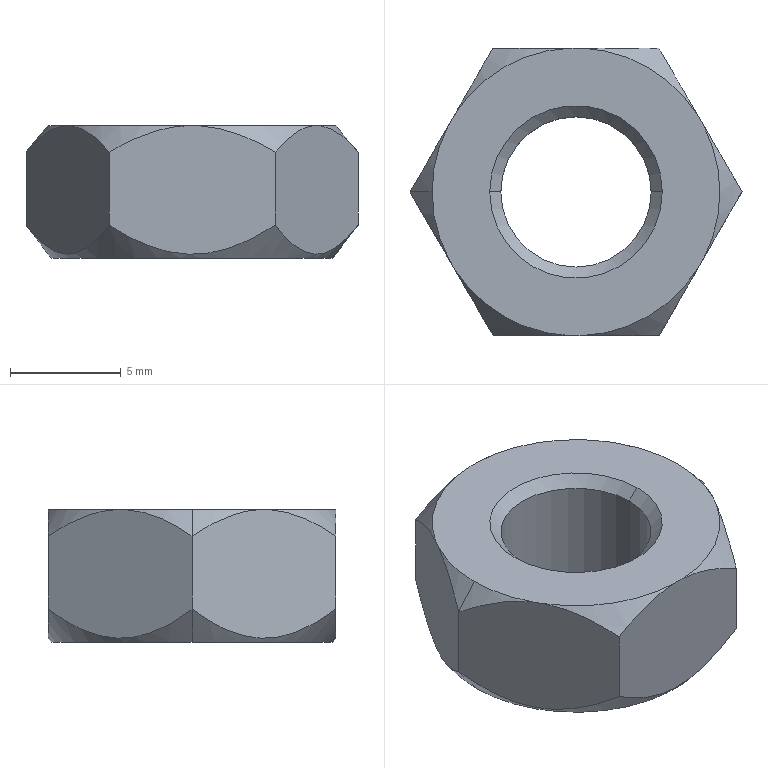Part | SolidWorks | features RevCut 3, Chamfer 2, Extrusion 1, RefAxis 1 | 1 solid | 23 faces | box 15.011 x 13.013 x 6 mm | volume 641.329 mm3 | cone 13 | plane 8 | cylinder 2 | commonest cylinder face diameters 6.8 x2
STEP:
#1=CARTESIAN_POINT('',(-3.4,0.,5.5));
#2=VERTEX_POINT('',#1);
#3=CARTESIAN_POINT('',(3.4,0.,5.5));
#4=VERTEX_POINT('',#3);
#5=CARTESIAN_POINT('',(0.,0.,5.5));
#6=DIRECTION('',(0.,0.,1.));
#7=DIRECTION('',(1.,0.,0.));
#8=AXIS2_PLACEMENT_3D('',#5,#6,#7);
#9=CIRCLE('',#8,3.4);
#10=EDGE_CURVE('',#2,#4,#9,.T.);
#11=ORIENTED_EDGE('',*,*,#10,.F.);
#12=CARTESIAN_POINT('',(-3.9,0.,6.));
#13=VERTEX_POINT('',#12);
#14=CARTESIAN_POINT('',(-3.4,0.,5.5));
#15=DIRECTION('',(-0.7071,0.,0.7071));
#16=VECTOR('',#15,1000.);
#17=LINE('',#14,#16);
#18=EDGE_CURVE('',#2,#13,#17,.T.);
#19=ORIENTED_EDGE('',*,*,#18,.T.);
#20=CARTESIAN_POINT('',(3.9,0.,6.));
#21=VERTEX_POINT('',#20);
#22=CARTESIAN_POINT('',(0.,0.,6.));
#23=DIRECTION('',(0.,0.,-1.));
#24=DIRECTION('',(1.,0.,0.));
#25=AXIS2_PLACEMENT_3D('',#22,#23,#24);
#26=CIRCLE('',#25,3.9);
#27=EDGE_CURVE('',#21,#13,#26,.T.);
#28=ORIENTED_EDGE('',*,*,#27,.F.);
#29=CARTESIAN_POINT('',(3.4,0.,5.5));
#30=DIRECTION('',(0.7071,0.,0.7071));
#31=VECTOR('',#30,1000.);
#32=LINE('',#29,#31);
#33=EDGE_CURVE('',#4,#21,#32,.T.);
#34=ORIENTED_EDGE('',*,*,#33,.F.);
#35=EDGE_LOOP('',(#11,#19,#28,#34));
#36=FACE_OUTER_BOUND('',#35,.T.);
#37=CARTESIAN_POINT('',(0.,0.,5.5));
#38=DIRECTION('',(0.,0.,1.));
#39=DIRECTION('',(1.,0.,0.));
#40=AXIS2_PLACEMENT_3D('',#37,#38,#39);
#41=CONICAL_SURFACE('',#40,3.4,0.7854);
#42=ADVANCED_FACE('',(#36),#41,.F.);
#43=CARTESIAN_POINT('',(3.4,0.,0.5));
#44=VERTEX_POINT('',#43);
#45=CARTESIAN_POINT('',(-3.4,0.,0.5));
#46=VERTEX_POINT('',#45);
#47=CARTESIAN_POINT('',(0.,0.,0.5));
#48=DIRECTION('',(0.,0.,-1.));
#49=DIRECTION('',(1.,0.,0.));
#50=AXIS2_PLACEMENT_3D('',#47,#48,#49);
#51=CIRCLE('',#50,3.4);
#52=EDGE_CURVE('',#44,#46,#51,.T.);
#53=ORIENTED_EDGE('',*,*,#52,.F.);
#54=CARTESIAN_POINT('',(3.9,0.,0.));
#55=VERTEX_POINT('',#54);
#56=CARTESIAN_POINT('',(3.9,0.,0.));
#57=DIRECTION('',(0.7071,0.,-0.7071));
#58=VECTOR('',#57,1000.);
#59=LINE('',#56,#58);
#60=EDGE_CURVE('',#44,#55,#59,.T.);
#61=ORIENTED_EDGE('',*,*,#60,.T.);
#62=CARTESIAN_POINT('',(-3.9,0.,0.));
#63=VERTEX_POINT('',#62);
#64=CARTESIAN_POINT('',(0.,0.,0.));
#65=DIRECTION('',(0.,0.,1.));
#66=DIRECTION('',(1.,0.,0.));
#67=AXIS2_PLACEMENT_3D('',#64,#65,#66);
#68=CIRCLE('',#67,3.9);
#69=EDGE_CURVE('',#63,#55,#68,.T.);
#70=ORIENTED_EDGE('',*,*,#69,.F.);
#71=CARTESIAN_POINT('',(-3.9,0.,0.));
#72=DIRECTION('',(-0.7071,0.,-0.7071));
#73=VECTOR('',#72,1000.);
#74=LINE('',#71,#73);
#75=EDGE_CURVE('',#46,#63,#74,.T.);
#76=ORIENTED_EDGE('',*,*,#75,.F.);
#77=EDGE_LOOP('',(#53,#61,#70,#76));
#78=FACE_OUTER_BOUND('',#77,.T.);
#79=CARTESIAN_POINT('',(0.,0.,0.));
#80=DIRECTION('',(0.,0.,-1.));
#81=DIRECTION('',(-1.,0.,0.));
#82=AXIS2_PLACEMENT_3D('',#79,#80,#81);
#83=CONICAL_SURFACE('',#82,3.9,0.7854);
#84=ADVANCED_FACE('',(#78),#83,.F.);
#85=CARTESIAN_POINT('',(-6.506,0.,6.));
#86=VERTEX_POINT('',#85);
#87=CARTESIAN_POINT('',(-5.758,-3.027,6.));
#88=VERTEX_POINT('',#87);
#89=CARTESIAN_POINT('',(0.,0.,6.));
#90=DIRECTION('',(0.,0.,1.));
#91=DIRECTION('',(1.,0.,0.));
#92=AXIS2_PLACEMENT_3D('',#89,#90,#91);
#93=CIRCLE('',#92,6.506);
#94=EDGE_CURVE('',#86,#88,#93,.T.);
#95=ORIENTED_EDGE('',*,*,#94,.F.);
#96=CARTESIAN_POINT('',(-7.498,0.,4.809));
#97=VERTEX_POINT('',#96);
#98=CARTESIAN_POINT('',(-6.506,0.,6.));
#99=DIRECTION('',(-0.6402,0.,-0.7682));
#100=VECTOR('',#99,1000.);
#101=LINE('',#98,#100);
#102=EDGE_CURVE('',#86,#97,#101,.T.);
#103=ORIENTED_EDGE('',*,*,#102,.T.);
#104=CARTESIAN_POINT('',(-7.506,-0.01301,4.8));
#105=VERTEX_POINT('',#104);
#106=CARTESIAN_POINT('',(-7.498,0.,4.809));
#107=CARTESIAN_POINT('',(-7.501,-0.004328,4.806));
#108=CARTESIAN_POINT('',(-7.503,-0.008655,4.803));
#109=CARTESIAN_POINT('',(-7.506,-0.01301,4.8));
#110=B_SPLINE_CURVE_WITH_KNOTS('',3,(#106,#107,#108,#109),.UNSPECIFIED.,.F.,.F.,(4,4),(0.01511,0.01513),.UNSPECIFIED.);
#111=EDGE_CURVE('',#97,#105,#110,.T.);
#112=ORIENTED_EDGE('',*,*,#111,.T.);
#113=CARTESIAN_POINT('',(-7.506,-0.01301,4.8));
#114=CARTESIAN_POINT('',(-7.373,-0.2423,4.959));
#115=CARTESIAN_POINT('',(-7.237,-0.4764,5.109));
#116=CARTESIAN_POINT('',(-6.958,-0.9577,5.384));
#117=CARTESIAN_POINT('',(-6.814,-1.206,5.509));
#118=CARTESIAN_POINT('',(-6.522,-1.71,5.723));
#119=CARTESIAN_POINT('',(-6.373,-1.966,5.811));
#120=CARTESIAN_POINT('',(-6.07,-2.489,5.942));
#121=CARTESIAN_POINT('',(-5.914,-2.759,5.985));
#122=CARTESIAN_POINT('',(-5.758,-3.027,6.));
#123=B_SPLINE_CURVE_WITH_KNOTS('',3,(#113,#114,#115,#116,#117,#118,#119,#120,#121,#122),.UNSPECIFIED.,.F.,.F.,(4,2,2,2,4),(0.007161,0.00809,0.00902,0.009949,0.01088),.UNSPECIFIED.);
#124=EDGE_CURVE('',#105,#88,#123,.T.);
#125=ORIENTED_EDGE('',*,*,#124,.T.);
#126=EDGE_LOOP('',(#95,#103,#112,#125));
#127=FACE_OUTER_BOUND('',#126,.T.);
#128=CARTESIAN_POINT('',(0.,0.,6.));
#129=DIRECTION('',(0.,0.,-1.));
#130=DIRECTION('',(-1.,0.,0.));
#131=AXIS2_PLACEMENT_3D('',#128,#129,#130);
#132=CONICAL_SURFACE('',#131,6.506,0.6947);
#133=ADVANCED_FACE('',(#127),#132,.T.);
#134=CARTESIAN_POINT('',(6.359,0.,0.));
#135=VERTEX_POINT('',#134);
#136=CARTESIAN_POINT('',(-6.359,0.,0.));
#137=VERTEX_POINT('',#136);
#138=CARTESIAN_POINT('',(0.,0.,0.));
#139=DIRECTION('',(0.,0.,1.));
#140=DIRECTION('',(1.,0.,0.));
#141=AXIS2_PLACEMENT_3D('',#138,#139,#140);
#142=CIRCLE('',#141,6.359);
#143=EDGE_CURVE('',#135,#137,#142,.T.);
#144=ORIENTED_EDGE('',*,*,#143,.T.);
#145=CARTESIAN_POINT('',(-7.498,0.,1.49));
#146=VERTEX_POINT('',#145);
#147=CARTESIAN_POINT('',(-7.506,0.,1.5));
#148=DIRECTION('',(-0.6074,0.,0.7944));
#149=VECTOR('',#148,1000.);
#150=LINE('',#147,#149);
#151=EDGE_CURVE('',#137,#146,#150,.T.);
#152=ORIENTED_EDGE('',*,*,#151,.T.);
#153=CARTESIAN_POINT('',(-3.764,6.493,1.5));
#154=VERTEX_POINT('',#153);
#155=CARTESIAN_POINT('',(-7.498,0.,1.49));
#156=CARTESIAN_POINT('',(-7.218,0.4875,1.124));
#157=CARTESIAN_POINT('',(-6.927,0.9929,0.8031));
#158=CARTESIAN_POINT('',(-6.463,1.8,0.4495));
#159=CARTESIAN_POINT('',(-6.303,2.079,0.3531));
#160=CARTESIAN_POINT('',(-5.972,2.654,0.22));
#161=CARTESIAN_POINT('',(-5.806,2.943,0.1855));
#162=CARTESIAN_POINT('',(-5.556,3.378,0.1847));
#163=CARTESIAN_POINT('',(-5.472,3.523,0.1928));
#164=CARTESIAN_POINT('',(-5.305,3.814,0.226));
#165=CARTESIAN_POINT('',(-5.221,3.96,0.2513));
#166=CARTESIAN_POINT('',(-4.974,4.39,0.3495));
#167=CARTESIAN_POINT('',(-4.814,4.668,0.4449));
#168=CARTESIAN_POINT('',(-4.5,5.214,0.6826));
#169=CARTESIAN_POINT('',(-4.346,5.481,0.8253));
#170=CARTESIAN_POINT('',(-4.049,5.997,1.141));
#171=CARTESIAN_POINT('',(-3.905,6.248,1.315));
#172=CARTESIAN_POINT('',(-3.764,6.493,1.5));
#173=B_SPLINE_CURVE_WITH_KNOTS('',3,(#155,#156,#157,#158,#159,#160,#161,#162,#163,#164,#165,#166,#167,#168,#169,#170,#171,#172),.UNSPECIFIED.,.F.,.F.,(4,2,2,2,2,2,2,2,4),(0.00001801,0.002007,0.003001,0.003996,0.004493,0.00499,0.005985,0.006979,0.007974),.UNSPECIFIED.);
#174=EDGE_CURVE('',#146,#154,#173,.T.);
#175=ORIENTED_EDGE('',*,*,#174,.T.);
#176=CARTESIAN_POINT('',(3.742,6.506,1.5));
#177=VERTEX_POINT('',#176);
#178=CARTESIAN_POINT('',(-3.764,6.493,1.5));
#179=CARTESIAN_POINT('',(-3.201,6.494,1.132));
#180=CARTESIAN_POINT('',(-2.617,6.495,0.8095));
#181=CARTESIAN_POINT('',(-1.684,6.497,0.4534));
#182=CARTESIAN_POINT('',(-1.363,6.498,0.3562));
#183=CARTESIAN_POINT('',(-0.6975,6.499,0.2214));
#184=CARTESIAN_POINT('',(-0.3636,6.499,0.1861));
#185=CARTESIAN_POINT('',(0.1388,6.5,0.1844));
#186=CARTESIAN_POINT('',(0.3066,6.501,0.1923));
#187=CARTESIAN_POINT('',(0.6427,6.501,0.225));
#188=CARTESIAN_POINT('',(0.8115,6.501,0.2501));
#189=CARTESIAN_POINT('',(1.309,6.502,0.3479));
#190=CARTESIAN_POINT('',(1.631,6.503,0.4433));
#191=CARTESIAN_POINT('',(2.262,6.504,0.681));
#192=CARTESIAN_POINT('',(2.571,6.504,0.824));
#193=CARTESIAN_POINT('',(3.168,6.506,1.141));
#194=CARTESIAN_POINT('',(3.458,6.506,1.315));
#195=CARTESIAN_POINT('',(3.742,6.506,1.5));
#196=B_SPLINE_CURVE_WITH_KNOTS('',3,(#178,#179,#180,#181,#182,#183,#184,#185,#186,#187,#188,#189,#190,#191,#192,#193,#194,#195),.UNSPECIFIED.,.F.,.F.,(4,2,2,2,2,2,2,2,4),(0.000000361,0.001994,0.00299,0.003987,0.004486,0.004984,0.005981,0.006977,0.007974),.UNSPECIFIED.);
#197=EDGE_CURVE('',#154,#177,#196,.T.);
#198=ORIENTED_EDGE('',*,*,#197,.T.);
#199=CARTESIAN_POINT('',(7.506,0.01301,1.5));
#200=VERTEX_POINT('',#199);
#201=CARTESIAN_POINT('',(3.742,6.506,1.5));
#202=CARTESIAN_POINT('',(4.024,6.019,1.132));
#203=CARTESIAN_POINT('',(4.317,5.514,0.8095));
#204=CARTESIAN_POINT('',(4.784,4.707,0.4534));
#205=CARTESIAN_POINT('',(4.946,4.429,0.3562));
#206=CARTESIAN_POINT('',(5.279,3.853,0.2214));
#207=CARTESIAN_POINT('',(5.447,3.565,0.1861));
#208=CARTESIAN_POINT('',(5.699,3.13,0.1844));
#209=CARTESIAN_POINT('',(5.783,2.985,0.1923));
#210=CARTESIAN_POINT('',(5.951,2.694,0.225));
#211=CARTESIAN_POINT('',(6.036,2.548,0.2501));
#212=CARTESIAN_POINT('',(6.286,2.118,0.3479));
#213=CARTESIAN_POINT('',(6.447,1.839,0.4433));
#214=CARTESIAN_POINT('',(6.763,1.293,0.681));
#215=CARTESIAN_POINT('',(6.918,1.026,0.824));
#216=CARTESIAN_POINT('',(7.218,0.5092,1.141));
#217=CARTESIAN_POINT('',(7.363,0.2584,1.315));
#218=CARTESIAN_POINT('',(7.506,0.01301,1.5));
#219=B_SPLINE_CURVE_WITH_KNOTS('',3,(#201,#202,#203,#204,#205,#206,#207,#208,#209,#210,#211,#212,#213,#214,#215,#216,#217,#218),.UNSPECIFIED.,.F.,.F.,(4,2,2,2,2,2,2,2,4),(0.000000361,0.001994,0.00299,0.003987,0.004486,0.004984,0.005981,0.006977,0.007974),.UNSPECIFIED.);
#220=EDGE_CURVE('',#177,#200,#219,.T.);
#221=ORIENTED_EDGE('',*,*,#220,.T.);
#222=CARTESIAN_POINT('',(7.498,0.,1.49));
#223=VERTEX_POINT('',#222);
#224=CARTESIAN_POINT('',(7.506,0.01301,1.5));
#225=CARTESIAN_POINT('',(7.503,0.008651,1.497));
#226=CARTESIAN_POINT('',(7.501,0.004326,1.493));
#227=CARTESIAN_POINT('',(7.498,0.,1.49));
#228=B_SPLINE_CURVE_WITH_KNOTS('',3,(#224,#225,#226,#227),.UNSPECIFIED.,.F.,.F.,(4,4),(0.000000361,0.00001801),.UNSPECIFIED.);
#229=EDGE_CURVE('',#200,#223,#228,.T.);
#230=ORIENTED_EDGE('',*,*,#229,.T.);
#231=CARTESIAN_POINT('',(7.506,0.,1.5));
#232=DIRECTION('',(0.6074,0.,0.7944));
#233=VECTOR('',#232,1000.);
#234=LINE('',#231,#233);
#235=EDGE_CURVE('',#135,#223,#234,.T.);
#236=ORIENTED_EDGE('',*,*,#235,.F.);
#237=EDGE_LOOP('',(#144,#152,#175,#198,#221,#230,#236));
#238=FACE_OUTER_BOUND('',#237,.T.);
#239=CARTESIAN_POINT('',(0.,0.,1.5));
#240=DIRECTION('',(0.,0.,1.));
#241=DIRECTION('',(1.,0.,0.));
#242=AXIS2_PLACEMENT_3D('',#239,#240,#241);
#243=CONICAL_SURFACE('',#242,7.506,0.6528);
#244=ADVANCED_FACE('',(#238),#243,.T.);
#245=ORIENTED_EDGE('',*,*,#10,.T.);
#246=CARTESIAN_POINT('',(3.4,0.,6.));
#247=DIRECTION('',(0.,0.,-1.));
#248=VECTOR('',#247,1000.);
#249=LINE('',#246,#248);
#250=EDGE_CURVE('',#4,#44,#249,.T.);
#251=ORIENTED_EDGE('',*,*,#250,.T.);
#252=ORIENTED_EDGE('',*,*,#52,.T.);
#253=CARTESIAN_POINT('',(-3.4,0.,6.));
#254=DIRECTION('',(0.,0.,-1.));
#255=VECTOR('',#254,1000.);
#256=LINE('',#253,#255);
#257=EDGE_CURVE('',#2,#46,#256,.T.);
#258=ORIENTED_EDGE('',*,*,#257,.F.);
#259=EDGE_LOOP('',(#245,#251,#252,#258));
#260=FACE_OUTER_BOUND('',#259,.T.);
#261=CARTESIAN_POINT('',(0.,0.,6.));
#262=DIRECTION('',(0.,0.,-1.));
#263=DIRECTION('',(-1.,0.,0.));
#264=AXIS2_PLACEMENT_3D('',#261,#262,#263);
#265=CYLINDRICAL_SURFACE('',#264,3.4);
#266=ADVANCED_FACE('',(#260),#265,.F.);
#267=ORIENTED_EDGE('',*,*,#124,.F.);
#268=CARTESIAN_POINT('',(-7.506,-0.01301,1.5));
#269=VERTEX_POINT('',#268);
#270=CARTESIAN_POINT('',(-7.506,-0.01301,6.));
#271=DIRECTION('',(0.,0.,-1.));
#272=VECTOR('',#271,1000.);
#273=LINE('',#270,#272);
#274=EDGE_CURVE('',#105,#269,#273,.T.);
#275=ORIENTED_EDGE('',*,*,#274,.T.);
#276=CARTESIAN_POINT('',(-3.742,-6.506,1.5));
#277=VERTEX_POINT('',#276);
#278=CARTESIAN_POINT('',(-3.742,-6.506,1.5));
#279=CARTESIAN_POINT('',(-4.024,-6.019,1.132));
#280=CARTESIAN_POINT('',(-4.317,-5.514,0.8095));
#281=CARTESIAN_POINT('',(-4.784,-4.707,0.4534));
#282=CARTESIAN_POINT('',(-4.946,-4.429,0.3562));
#283=CARTESIAN_POINT('',(-5.279,-3.853,0.2214));
#284=CARTESIAN_POINT('',(-5.447,-3.565,0.1861));
#285=CARTESIAN_POINT('',(-5.699,-3.13,0.1844));
#286=CARTESIAN_POINT('',(-5.783,-2.985,0.1923));
#287=CARTESIAN_POINT('',(-5.951,-2.694,0.225));
#288=CARTESIAN_POINT('',(-6.036,-2.548,0.2501));
#289=CARTESIAN_POINT('',(-6.286,-2.118,0.3479));
#290=CARTESIAN_POINT('',(-6.447,-1.839,0.4433));
#291=CARTESIAN_POINT('',(-6.763,-1.293,0.681));
#292=CARTESIAN_POINT('',(-6.918,-1.026,0.824));
#293=CARTESIAN_POINT('',(-7.218,-0.5092,1.141));
#294=CARTESIAN_POINT('',(-7.363,-0.2584,1.315));
#295=CARTESIAN_POINT('',(-7.506,-0.01301,1.5));
#296=B_SPLINE_CURVE_WITH_KNOTS('',3,(#278,#279,#280,#281,#282,#283,#284,#285,#286,#287,#288,#289,#290,#291,#292,#293,#294,#295),.UNSPECIFIED.,.F.,.F.,(4,2,2,2,2,2,2,2,4),(0.000000361,0.001994,0.00299,0.003987,0.004486,0.004984,0.005981,0.006977,0.007974),.UNSPECIFIED.);
#297=EDGE_CURVE('',#277,#269,#296,.T.);
#298=ORIENTED_EDGE('',*,*,#297,.F.);
#299=CARTESIAN_POINT('',(-3.742,-6.506,4.8));
#300=VERTEX_POINT('',#299);
#301=CARTESIAN_POINT('',(-3.742,-6.506,6.));
#302=DIRECTION('',(0.,0.,-1.));
#303=VECTOR('',#302,1000.);
#304=LINE('',#301,#303);
#305=EDGE_CURVE('',#300,#277,#304,.T.);
#306=ORIENTED_EDGE('',*,*,#305,.F.);
#307=CARTESIAN_POINT('',(-5.489,-3.492,6.));
#308=VERTEX_POINT('',#307);
#309=CARTESIAN_POINT('',(-5.489,-3.492,6.));
#310=CARTESIAN_POINT('',(-5.334,-3.759,5.985));
#311=CARTESIAN_POINT('',(-5.18,-4.024,5.943));
#312=CARTESIAN_POINT('',(-4.875,-4.55,5.812));
#313=CARTESIAN_POINT('',(-4.724,-4.812,5.722));
#314=CARTESIAN_POINT('',(-4.285,-5.568,5.401));
#315=CARTESIAN_POINT('',(-4.009,-6.045,5.12));
#316=CARTESIAN_POINT('',(-3.742,-6.506,4.8));
#317=B_SPLINE_CURVE_WITH_KNOTS('',3,(#309,#310,#311,#312,#313,#314,#315,#316),.UNSPECIFIED.,.F.,.F.,(4,2,2,4),(0.01142,0.01235,0.01328,0.01515),.UNSPECIFIED.);
#318=EDGE_CURVE('',#308,#300,#317,.T.);
#319=ORIENTED_EDGE('',*,*,#318,.F.);
#320=CARTESIAN_POINT('',(-7.506,-0.01301,6.));
#321=DIRECTION('',(0.5015,-0.8652,0.));
#322=VECTOR('',#321,1000.);
#323=LINE('',#320,#322);
#324=EDGE_CURVE('',#88,#308,#323,.T.);
#325=ORIENTED_EDGE('',*,*,#324,.F.);
#326=EDGE_LOOP('',(#267,#275,#298,#306,#319,#325));
#327=FACE_OUTER_BOUND('',#326,.T.);
#328=CARTESIAN_POINT('',(-7.506,-0.01301,6.));
#329=DIRECTION('',(0.8652,0.5015,0.));
#330=DIRECTION('',(-0.5015,0.8652,0.));
#331=AXIS2_PLACEMENT_3D('',#328,#329,#330);
#332=PLANE('',#331);
#333=ADVANCED_FACE('',(#327),#332,.F.);
#334=CARTESIAN_POINT('',(-0.2572,-6.5,6.));
#335=VERTEX_POINT('',#334);
#336=CARTESIAN_POINT('',(-3.742,-6.506,4.8));
#337=CARTESIAN_POINT('',(-3.207,-6.506,5.12));
#338=CARTESIAN_POINT('',(-2.655,-6.505,5.402));
#339=CARTESIAN_POINT('',(-1.78,-6.503,5.723));
#340=CARTESIAN_POINT('',(-1.478,-6.503,5.812));
#341=CARTESIAN_POINT('',(-0.8727,-6.502,5.943));
#342=CARTESIAN_POINT('',(-0.5667,-6.501,5.985));
#343=CARTESIAN_POINT('',(-0.2572,-6.5,6.));
#344=B_SPLINE_CURVE_WITH_KNOTS('',3,(#336,#337,#338,#339,#340,#341,#342,#343),.UNSPECIFIED.,.F.,.F.,(4,2,2,4),(0.005934,0.007788,0.008715,0.009642),.UNSPECIFIED.);
#345=EDGE_CURVE('',#300,#335,#344,.T.);
#346=ORIENTED_EDGE('',*,*,#345,.F.);
#347=ORIENTED_EDGE('',*,*,#305,.T.);
#348=CARTESIAN_POINT('',(3.764,-6.493,1.5));
#349=VERTEX_POINT('',#348);
#350=CARTESIAN_POINT('',(3.764,-6.493,1.5));
#351=CARTESIAN_POINT('',(3.201,-6.494,1.132));
#352=CARTESIAN_POINT('',(2.617,-6.495,0.8095));
#353=CARTESIAN_POINT('',(1.684,-6.497,0.4534));
#354=CARTESIAN_POINT('',(1.363,-6.498,0.3562));
#355=CARTESIAN_POINT('',(0.6975,-6.499,0.2214));
#356=CARTESIAN_POINT('',(0.3636,-6.499,0.1861));
#357=CARTESIAN_POINT('',(-0.1388,-6.5,0.1844));
#358=CARTESIAN_POINT('',(-0.3066,-6.501,0.1923));
#359=CARTESIAN_POINT('',(-0.6427,-6.501,0.225));
#360=CARTESIAN_POINT('',(-0.8115,-6.501,0.2501));
#361=CARTESIAN_POINT('',(-1.309,-6.502,0.3479));
#362=CARTESIAN_POINT('',(-1.631,-6.503,0.4433));
#363=CARTESIAN_POINT('',(-2.262,-6.504,0.681));
#364=CARTESIAN_POINT('',(-2.571,-6.504,0.824));
#365=CARTESIAN_POINT('',(-3.168,-6.506,1.141));
#366=CARTESIAN_POINT('',(-3.458,-6.506,1.315));
#367=CARTESIAN_POINT('',(-3.742,-6.506,1.5));
#368=B_SPLINE_CURVE_WITH_KNOTS('',3,(#350,#351,#352,#353,#354,#355,#356,#357,#358,#359,#360,#361,#362,#363,#364,#365,#366,#367),.UNSPECIFIED.,.F.,.F.,(4,2,2,2,2,2,2,2,4),(0.000000361,0.001994,0.00299,0.003987,0.004486,0.004984,0.005981,0.006977,0.007974),.UNSPECIFIED.);
#369=EDGE_CURVE('',#349,#277,#368,.T.);
#370=ORIENTED_EDGE('',*,*,#369,.F.);
#371=CARTESIAN_POINT('',(3.764,-6.493,4.8));
#372=VERTEX_POINT('',#371);
#373=CARTESIAN_POINT('',(3.764,-6.493,6.));
#374=DIRECTION('',(0.,0.,-1.));
#375=VECTOR('',#374,1000.);
#376=LINE('',#373,#375);
#377=EDGE_CURVE('',#372,#349,#376,.T.);
#378=ORIENTED_EDGE('',*,*,#377,.F.);
#379=CARTESIAN_POINT('',(0.2797,-6.5,6.));
#380=VERTEX_POINT('',#379);
#381=CARTESIAN_POINT('',(0.2797,-6.5,6.));
#382=CARTESIAN_POINT('',(0.9057,-6.498,5.969));
#383=CARTESIAN_POINT('',(1.509,-6.497,5.83));
#384=CARTESIAN_POINT('',(2.684,-6.495,5.4));
#385=CARTESIAN_POINT('',(3.234,-6.494,5.118));
#386=CARTESIAN_POINT('',(3.764,-6.493,4.8));
#387=B_SPLINE_CURVE_WITH_KNOTS('',3,(#381,#382,#383,#384,#385,#386),.UNSPECIFIED.,.F.,.F.,(4,2,4),(0.01017,0.01203,0.01389),.UNSPECIFIED.);
#388=EDGE_CURVE('',#380,#372,#387,.T.);
#389=ORIENTED_EDGE('',*,*,#388,.F.);
#390=CARTESIAN_POINT('',(-3.742,-6.506,6.));
#391=DIRECTION('',(1.,0.001733,0.));
#392=VECTOR('',#391,1000.);
#393=LINE('',#390,#392);
#394=EDGE_CURVE('',#335,#380,#393,.T.);
#395=ORIENTED_EDGE('',*,*,#394,.F.);
#396=EDGE_LOOP('',(#346,#347,#370,#378,#389,#395));
#397=FACE_OUTER_BOUND('',#396,.T.);
#398=CARTESIAN_POINT('',(-3.742,-6.506,6.));
#399=DIRECTION('',(-0.001733,1.,0.));
#400=DIRECTION('',(-1.,-0.001733,0.));
#401=AXIS2_PLACEMENT_3D('',#398,#399,#400);
#402=PLANE('',#401);
#403=ADVANCED_FACE('',(#397),#402,.F.);
#404=CARTESIAN_POINT('',(5.501,-3.473,6.));
#405=VERTEX_POINT('',#404);
#406=CARTESIAN_POINT('',(3.764,-6.493,4.8));
#407=CARTESIAN_POINT('',(3.896,-6.264,4.959));
#408=CARTESIAN_POINT('',(4.031,-6.029,5.109));
#409=CARTESIAN_POINT('',(4.308,-5.547,5.384));
#410=CARTESIAN_POINT('',(4.452,-5.298,5.509));
#411=CARTESIAN_POINT('',(4.742,-4.793,5.723));
#412=CARTESIAN_POINT('',(4.889,-4.536,5.811));
#413=CARTESIAN_POINT('',(5.191,-4.012,5.942));
#414=CARTESIAN_POINT('',(5.346,-3.742,5.985));
#415=CARTESIAN_POINT('',(5.501,-3.473,6.));
#416=B_SPLINE_CURVE_WITH_KNOTS('',3,(#406,#407,#408,#409,#410,#411,#412,#413,#414,#415),.UNSPECIFIED.,.F.,.F.,(4,2,2,2,4),(0.007144,0.008073,0.009002,0.009932,0.01086),.UNSPECIFIED.);
#417=EDGE_CURVE('',#372,#405,#416,.T.);
#418=ORIENTED_EDGE('',*,*,#417,.F.);
#419=ORIENTED_EDGE('',*,*,#377,.T.);
#420=CARTESIAN_POINT('',(7.498,0.,1.49));
#421=CARTESIAN_POINT('',(7.218,-0.4875,1.124));
#422=CARTESIAN_POINT('',(6.927,-0.9929,0.8031));
#423=CARTESIAN_POINT('',(6.463,-1.8,0.4495));
#424=CARTESIAN_POINT('',(6.303,-2.079,0.3531));
#425=CARTESIAN_POINT('',(5.972,-2.654,0.22));
#426=CARTESIAN_POINT('',(5.806,-2.943,0.1855));
#427=CARTESIAN_POINT('',(5.556,-3.378,0.1847));
#428=CARTESIAN_POINT('',(5.472,-3.523,0.1928));
#429=CARTESIAN_POINT('',(5.305,-3.814,0.226));
#430=CARTESIAN_POINT('',(5.221,-3.96,0.2513));
#431=CARTESIAN_POINT('',(4.974,-4.39,0.3495));
#432=CARTESIAN_POINT('',(4.814,-4.668,0.4449));
#433=CARTESIAN_POINT('',(4.5,-5.214,0.6826));
#434=CARTESIAN_POINT('',(4.346,-5.481,0.8253));
#435=CARTESIAN_POINT('',(4.049,-5.997,1.141));
#436=CARTESIAN_POINT('',(3.905,-6.248,1.315));
#437=CARTESIAN_POINT('',(3.764,-6.493,1.5));
#438=B_SPLINE_CURVE_WITH_KNOTS('',3,(#420,#421,#422,#423,#424,#425,#426,#427,#428,#429,#430,#431,#432,#433,#434,#435,#436,#437),.UNSPECIFIED.,.F.,.F.,(4,2,2,2,2,2,2,2,4),(0.00001801,0.002007,0.003001,0.003996,0.004493,0.00499,0.005985,0.006979,0.007974),.UNSPECIFIED.);
#439=EDGE_CURVE('',#223,#349,#438,.T.);
#440=ORIENTED_EDGE('',*,*,#439,.F.);
#441=ORIENTED_EDGE('',*,*,#229,.F.);
#442=CARTESIAN_POINT('',(7.506,0.01301,4.8));
#443=VERTEX_POINT('',#442);
#444=CARTESIAN_POINT('',(7.506,0.01301,6.));
#445=DIRECTION('',(0.,0.,-1.));
#446=VECTOR('',#445,1000.);
#447=LINE('',#444,#446);
#448=EDGE_CURVE('',#443,#200,#447,.T.);
#449=ORIENTED_EDGE('',*,*,#448,.F.);
#450=CARTESIAN_POINT('',(5.769,-3.007,6.));
#451=VERTEX_POINT('',#450);
#452=CARTESIAN_POINT('',(5.769,-3.007,6.));
#453=CARTESIAN_POINT('',(5.923,-2.74,5.985));
#454=CARTESIAN_POINT('',(6.075,-2.474,5.943));
#455=CARTESIAN_POINT('',(6.378,-1.947,5.812));
#456=CARTESIAN_POINT('',(6.529,-1.685,5.722));
#457=CARTESIAN_POINT('',(6.965,-0.9271,5.401));
#458=CARTESIAN_POINT('',(7.24,-0.4492,5.12));
#459=CARTESIAN_POINT('',(7.506,0.01301,4.8));
#460=B_SPLINE_CURVE_WITH_KNOTS('',3,(#452,#453,#454,#455,#456,#457,#458,#459),.UNSPECIFIED.,.F.,.F.,(4,2,2,4),(0.0114,0.01233,0.01326,0.01513),.UNSPECIFIED.);
#461=EDGE_CURVE('',#451,#443,#460,.T.);
#462=ORIENTED_EDGE('',*,*,#461,.F.);
#463=CARTESIAN_POINT('',(3.764,-6.493,6.));
#464=DIRECTION('',(0.4985,0.8669,0.));
#465=VECTOR('',#464,1000.);
#466=LINE('',#463,#465);
#467=EDGE_CURVE('',#405,#451,#466,.T.);
#468=ORIENTED_EDGE('',*,*,#467,.F.);
#469=EDGE_LOOP('',(#418,#419,#440,#441,#449,#462,#468));
#470=FACE_OUTER_BOUND('',#469,.T.);
#471=CARTESIAN_POINT('',(3.764,-6.493,6.));
#472=DIRECTION('',(-0.8669,0.4985,0.));
#473=DIRECTION('',(-0.4985,-0.8669,0.));
#474=AXIS2_PLACEMENT_3D('',#471,#472,#473);
#475=PLANE('',#474);
#476=ADVANCED_FACE('',(#470),#475,.F.);
#477=CARTESIAN_POINT('',(5.758,3.027,6.));
#478=VERTEX_POINT('',#477);
#479=CARTESIAN_POINT('',(7.506,0.01301,4.8));
#480=CARTESIAN_POINT('',(7.373,0.2423,4.959));
#481=CARTESIAN_POINT('',(7.237,0.4764,5.109));
#482=CARTESIAN_POINT('',(6.958,0.9577,5.384));
#483=CARTESIAN_POINT('',(6.814,1.206,5.509));
#484=CARTESIAN_POINT('',(6.522,1.71,5.723));
#485=CARTESIAN_POINT('',(6.373,1.966,5.811));
#486=CARTESIAN_POINT('',(6.07,2.489,5.942));
#487=CARTESIAN_POINT('',(5.914,2.759,5.985));
#488=CARTESIAN_POINT('',(5.758,3.027,6.));
#489=B_SPLINE_CURVE_WITH_KNOTS('',3,(#479,#480,#481,#482,#483,#484,#485,#486,#487,#488),.UNSPECIFIED.,.F.,.F.,(4,2,2,2,4),(0.007161,0.00809,0.00902,0.009949,0.01088),.UNSPECIFIED.);
#490=EDGE_CURVE('',#443,#478,#489,.T.);
#491=ORIENTED_EDGE('',*,*,#490,.F.);
#492=ORIENTED_EDGE('',*,*,#448,.T.);
#493=ORIENTED_EDGE('',*,*,#220,.F.);
#494=CARTESIAN_POINT('',(3.742,6.506,4.8));
#495=VERTEX_POINT('',#494);
#496=CARTESIAN_POINT('',(3.742,6.506,6.));
#497=DIRECTION('',(0.,0.,-1.));
#498=VECTOR('',#497,1000.);
#499=LINE('',#496,#498);
#500=EDGE_CURVE('',#495,#177,#499,.T.);
#501=ORIENTED_EDGE('',*,*,#500,.F.);
#502=CARTESIAN_POINT('',(5.489,3.492,6.));
#503=VERTEX_POINT('',#502);
#504=CARTESIAN_POINT('',(5.489,3.492,6.));
#505=CARTESIAN_POINT('',(5.334,3.759,5.985));
#506=CARTESIAN_POINT('',(5.18,4.024,5.943));
#507=CARTESIAN_POINT('',(4.875,4.55,5.812));
#508=CARTESIAN_POINT('',(4.724,4.812,5.722));
#509=CARTESIAN_POINT('',(4.285,5.568,5.401));
#510=CARTESIAN_POINT('',(4.009,6.045,5.12));
#511=CARTESIAN_POINT('',(3.742,6.506,4.8));
#512=B_SPLINE_CURVE_WITH_KNOTS('',3,(#504,#505,#506,#507,#508,#509,#510,#511),.UNSPECIFIED.,.F.,.F.,(4,2,2,4),(0.01142,0.01235,0.01328,0.01515),.UNSPECIFIED.);
#513=EDGE_CURVE('',#503,#495,#512,.T.);
#514=ORIENTED_EDGE('',*,*,#513,.F.);
#515=CARTESIAN_POINT('',(7.506,0.01301,6.));
#516=DIRECTION('',(-0.5015,0.8652,0.));
#517=VECTOR('',#516,1000.);
#518=LINE('',#515,#517);
#519=EDGE_CURVE('',#478,#503,#518,.T.);
#520=ORIENTED_EDGE('',*,*,#519,.F.);
#521=EDGE_LOOP('',(#491,#492,#493,#501,#514,#520));
#522=FACE_OUTER_BOUND('',#521,.T.);
#523=CARTESIAN_POINT('',(7.506,0.01301,6.));
#524=DIRECTION('',(-0.8652,-0.5015,0.));
#525=DIRECTION('',(0.5015,-0.8652,0.));
#526=AXIS2_PLACEMENT_3D('',#523,#524,#525);
#527=PLANE('',#526);
#528=ADVANCED_FACE('',(#522),#527,.F.);
#529=CARTESIAN_POINT('',(0.2572,6.5,6.));
#530=VERTEX_POINT('',#529);
#531=CARTESIAN_POINT('',(3.742,6.506,4.8));
#532=CARTESIAN_POINT('',(3.207,6.506,5.12));
#533=CARTESIAN_POINT('',(2.655,6.505,5.402));
#534=CARTESIAN_POINT('',(1.78,6.503,5.723));
#535=CARTESIAN_POINT('',(1.478,6.503,5.812));
#536=CARTESIAN_POINT('',(0.8727,6.502,5.943));
#537=CARTESIAN_POINT('',(0.5667,6.501,5.985));
#538=CARTESIAN_POINT('',(0.2572,6.5,6.));
#539=B_SPLINE_CURVE_WITH_KNOTS('',3,(#531,#532,#533,#534,#535,#536,#537,#538),.UNSPECIFIED.,.F.,.F.,(4,2,2,4),(0.005934,0.007788,0.008715,0.009642),.UNSPECIFIED.);
#540=EDGE_CURVE('',#495,#530,#539,.T.);
#541=ORIENTED_EDGE('',*,*,#540,.F.);
#542=ORIENTED_EDGE('',*,*,#500,.T.);
#543=ORIENTED_EDGE('',*,*,#197,.F.);
#544=CARTESIAN_POINT('',(-3.764,6.493,4.8));
#545=VERTEX_POINT('',#544);
#546=CARTESIAN_POINT('',(-3.764,6.493,6.));
#547=DIRECTION('',(0.,0.,-1.));
#548=VECTOR('',#547,1000.);
#549=LINE('',#546,#548);
#550=EDGE_CURVE('',#545,#154,#549,.T.);
#551=ORIENTED_EDGE('',*,*,#550,.F.);
#552=CARTESIAN_POINT('',(-0.2797,6.5,6.));
#553=VERTEX_POINT('',#552);
#554=CARTESIAN_POINT('',(-0.2797,6.5,6.));
#555=CARTESIAN_POINT('',(-0.9057,6.498,5.969));
#556=CARTESIAN_POINT('',(-1.509,6.497,5.83));
#557=CARTESIAN_POINT('',(-2.684,6.495,5.4));
#558=CARTESIAN_POINT('',(-3.234,6.494,5.118));
#559=CARTESIAN_POINT('',(-3.764,6.493,4.8));
#560=B_SPLINE_CURVE_WITH_KNOTS('',3,(#554,#555,#556,#557,#558,#559),.UNSPECIFIED.,.F.,.F.,(4,2,4),(0.01017,0.01203,0.01389),.UNSPECIFIED.);
#561=EDGE_CURVE('',#553,#545,#560,.T.);
#562=ORIENTED_EDGE('',*,*,#561,.F.);
#563=CARTESIAN_POINT('',(3.742,6.506,6.));
#564=DIRECTION('',(-1.,-0.001733,0.));
#565=VECTOR('',#564,1000.);
#566=LINE('',#563,#565);
#567=EDGE_CURVE('',#530,#553,#566,.T.);
#568=ORIENTED_EDGE('',*,*,#567,.F.);
#569=EDGE_LOOP('',(#541,#542,#543,#551,#562,#568));
#570=FACE_OUTER_BOUND('',#569,.T.);
#571=CARTESIAN_POINT('',(3.742,6.506,6.));
#572=DIRECTION('',(0.001733,-1.,0.));
#573=DIRECTION('',(1.,0.001733,0.));
#574=AXIS2_PLACEMENT_3D('',#571,#572,#573);
#575=PLANE('',#574);
#576=ADVANCED_FACE('',(#570),#575,.F.);
#577=CARTESIAN_POINT('',(-5.501,3.473,6.));
#578=VERTEX_POINT('',#577);
#579=CARTESIAN_POINT('',(-3.764,6.493,4.8));
#580=CARTESIAN_POINT('',(-3.896,6.264,4.959));
#581=CARTESIAN_POINT('',(-4.031,6.029,5.109));
#582=CARTESIAN_POINT('',(-4.308,5.547,5.384));
#583=CARTESIAN_POINT('',(-4.452,5.298,5.509));
#584=CARTESIAN_POINT('',(-4.742,4.793,5.723));
#585=CARTESIAN_POINT('',(-4.889,4.536,5.811));
#586=CARTESIAN_POINT('',(-5.191,4.012,5.942));
#587=CARTESIAN_POINT('',(-5.346,3.742,5.985));
#588=CARTESIAN_POINT('',(-5.501,3.473,6.));
#589=B_SPLINE_CURVE_WITH_KNOTS('',3,(#579,#580,#581,#582,#583,#584,#585,#586,#587,#588),.UNSPECIFIED.,.F.,.F.,(4,2,2,2,4),(0.007144,0.008073,0.009002,0.009932,0.01086),.UNSPECIFIED.);
#590=EDGE_CURVE('',#545,#578,#589,.T.);
#591=ORIENTED_EDGE('',*,*,#590,.F.);
#592=ORIENTED_EDGE('',*,*,#550,.T.);
#593=ORIENTED_EDGE('',*,*,#174,.F.);
#594=CARTESIAN_POINT('',(-7.506,-0.01301,1.5));
#595=CARTESIAN_POINT('',(-7.503,-0.008651,1.497));
#596=CARTESIAN_POINT('',(-7.501,-0.004326,1.493));
#597=CARTESIAN_POINT('',(-7.498,0.,1.49));
#598=B_SPLINE_CURVE_WITH_KNOTS('',3,(#594,#595,#596,#597),.UNSPECIFIED.,.F.,.F.,(4,4),(0.000000361,0.00001801),.UNSPECIFIED.);
#599=EDGE_CURVE('',#269,#146,#598,.T.);
#600=ORIENTED_EDGE('',*,*,#599,.F.);
#601=ORIENTED_EDGE('',*,*,#274,.F.);
#602=ORIENTED_EDGE('',*,*,#111,.F.);
#603=CARTESIAN_POINT('',(-5.769,3.007,6.));
#604=VERTEX_POINT('',#603);
#605=CARTESIAN_POINT('',(-5.769,3.007,6.));
#606=CARTESIAN_POINT('',(-5.922,2.741,5.985));
#607=CARTESIAN_POINT('',(-6.074,2.477,5.944));
#608=CARTESIAN_POINT('',(-6.376,1.952,5.813));
#609=CARTESIAN_POINT('',(-6.526,1.691,5.724));
#610=CARTESIAN_POINT('',(-6.96,0.9363,5.406));
#611=CARTESIAN_POINT('',(-7.233,0.4604,5.127));
#612=CARTESIAN_POINT('',(-7.498,0.,4.809));
#613=B_SPLINE_CURVE_WITH_KNOTS('',3,(#605,#606,#607,#608,#609,#610,#611,#612),.UNSPECIFIED.,.F.,.F.,(4,2,2,4),(0.0114,0.01233,0.01326,0.01511),.UNSPECIFIED.);
#614=EDGE_CURVE('',#604,#97,#613,.T.);
#615=ORIENTED_EDGE('',*,*,#614,.F.);
#616=CARTESIAN_POINT('',(-3.764,6.493,6.));
#617=DIRECTION('',(-0.4985,-0.8669,0.));
#618=VECTOR('',#617,1000.);
#619=LINE('',#616,#618);
#620=EDGE_CURVE('',#578,#604,#619,.T.);
#621=ORIENTED_EDGE('',*,*,#620,.F.);
#622=EDGE_LOOP('',(#591,#592,#593,#600,#601,#602,#615,#621));
#623=FACE_OUTER_BOUND('',#622,.T.);
#624=CARTESIAN_POINT('',(-3.764,6.493,6.));
#625=DIRECTION('',(0.8669,-0.4985,0.));
#626=DIRECTION('',(0.4985,0.8669,0.));
#627=AXIS2_PLACEMENT_3D('',#624,#625,#626);
#628=PLANE('',#627);
#629=ADVANCED_FACE('',(#623),#628,.F.);
#630=ORIENTED_EDGE('',*,*,#27,.T.);
#631=CARTESIAN_POINT('',(0.,0.,6.));
#632=DIRECTION('',(0.,0.,-1.));
#633=DIRECTION('',(1.,0.,0.));
#634=AXIS2_PLACEMENT_3D('',#631,#632,#633);
#635=CIRCLE('',#634,3.9);
#636=EDGE_CURVE('',#13,#21,#635,.T.);
#637=ORIENTED_EDGE('',*,*,#636,.T.);
#638=EDGE_LOOP('',(#630,#637));
#639=FACE_BOUND('',#638,.T.);
#640=ORIENTED_EDGE('',*,*,#519,.T.);
#641=CARTESIAN_POINT('',(0.,0.,6.));
#642=DIRECTION('',(0.,0.,1.));
#643=DIRECTION('',(1.,0.,0.));
#644=AXIS2_PLACEMENT_3D('',#641,#642,#643);
#645=CIRCLE('',#644,6.506);
#646=EDGE_CURVE('',#503,#530,#645,.T.);
#647=ORIENTED_EDGE('',*,*,#646,.T.);
#648=ORIENTED_EDGE('',*,*,#567,.T.);
#649=CARTESIAN_POINT('',(0.,0.,6.));
#650=DIRECTION('',(0.,0.,1.));
#651=DIRECTION('',(1.,0.,0.));
#652=AXIS2_PLACEMENT_3D('',#649,#650,#651);
#653=CIRCLE('',#652,6.506);
#654=EDGE_CURVE('',#553,#578,#653,.T.);
#655=ORIENTED_EDGE('',*,*,#654,.T.);
#656=ORIENTED_EDGE('',*,*,#620,.T.);
#657=CARTESIAN_POINT('',(0.,0.,6.));
#658=DIRECTION('',(0.,0.,1.));
#659=DIRECTION('',(1.,0.,0.));
#660=AXIS2_PLACEMENT_3D('',#657,#658,#659);
#661=CIRCLE('',#660,6.506);
#662=EDGE_CURVE('',#604,#86,#661,.T.);
#663=ORIENTED_EDGE('',*,*,#662,.T.);
#664=ORIENTED_EDGE('',*,*,#94,.T.);
#665=ORIENTED_EDGE('',*,*,#324,.T.);
#666=CARTESIAN_POINT('',(0.,0.,6.));
#667=DIRECTION('',(0.,0.,1.));
#668=DIRECTION('',(1.,0.,0.));
#669=AXIS2_PLACEMENT_3D('',#666,#667,#668);
#670=CIRCLE('',#669,6.506);
#671=EDGE_CURVE('',#308,#335,#670,.T.);
#672=ORIENTED_EDGE('',*,*,#671,.T.);
#673=ORIENTED_EDGE('',*,*,#394,.T.);
#674=CARTESIAN_POINT('',(0.,0.,6.));
#675=DIRECTION('',(0.,0.,1.));
#676=DIRECTION('',(1.,0.,0.));
#677=AXIS2_PLACEMENT_3D('',#674,#675,#676);
#678=CIRCLE('',#677,6.506);
#679=EDGE_CURVE('',#380,#405,#678,.T.);
#680=ORIENTED_EDGE('',*,*,#679,.T.);
#681=ORIENTED_EDGE('',*,*,#467,.T.);
#682=CARTESIAN_POINT('',(0.,0.,6.));
#683=DIRECTION('',(0.,0.,1.));
#684=DIRECTION('',(1.,0.,0.));
#685=AXIS2_PLACEMENT_3D('',#682,#683,#684);
#686=CIRCLE('',#685,6.506);
#687=EDGE_CURVE('',#451,#478,#686,.T.);
#688=ORIENTED_EDGE('',*,*,#687,.T.);
#689=EDGE_LOOP('',(#640,#647,#648,#655,#656,#663,#664,#665,#672,#673,#680,#681,#688));
#690=FACE_OUTER_BOUND('',#689,.T.);
#691=CARTESIAN_POINT('',(0.,0.,6.));
#692=DIRECTION('',(0.,0.,1.));
#693=DIRECTION('',(1.,0.,0.));
#694=AXIS2_PLACEMENT_3D('',#691,#692,#693);
#695=PLANE('',#694);
#696=ADVANCED_FACE('',(#639,#690),#695,.T.);
#697=ORIENTED_EDGE('',*,*,#69,.T.);
#698=CARTESIAN_POINT('',(0.,0.,0.));
#699=DIRECTION('',(0.,0.,1.));
#700=DIRECTION('',(1.,0.,0.));
#701=AXIS2_PLACEMENT_3D('',#698,#699,#700);
#702=CIRCLE('',#701,3.9);
#703=EDGE_CURVE('',#55,#63,#702,.T.);
#704=ORIENTED_EDGE('',*,*,#703,.T.);
#705=EDGE_LOOP('',(#697,#704));
#706=FACE_BOUND('',#705,.T.);
#707=ORIENTED_EDGE('',*,*,#143,.F.);
#708=CARTESIAN_POINT('',(0.,0.,0.));
#709=DIRECTION('',(0.,0.,1.));
#710=DIRECTION('',(1.,0.,0.));
#711=AXIS2_PLACEMENT_3D('',#708,#709,#710);
#712=CIRCLE('',#711,6.359);
#713=EDGE_CURVE('',#137,#135,#712,.T.);
#714=ORIENTED_EDGE('',*,*,#713,.F.);
#715=EDGE_LOOP('',(#707,#714));
#716=FACE_OUTER_BOUND('',#715,.T.);
#717=CARTESIAN_POINT('',(0.,0.,0.));
#718=DIRECTION('',(0.,0.,1.));
#719=DIRECTION('',(1.,0.,0.));
#720=AXIS2_PLACEMENT_3D('',#717,#718,#719);
#721=PLANE('',#720);
#722=ADVANCED_FACE('',(#706,#716),#721,.F.);
#723=ORIENTED_EDGE('',*,*,#250,.F.);
#724=CARTESIAN_POINT('',(0.,0.,5.5));
#725=DIRECTION('',(0.,0.,1.));
#726=DIRECTION('',(1.,0.,0.));
#727=AXIS2_PLACEMENT_3D('',#724,#725,#726);
#728=CIRCLE('',#727,3.4);
#729=EDGE_CURVE('',#4,#2,#728,.T.);
#730=ORIENTED_EDGE('',*,*,#729,.T.);
#731=ORIENTED_EDGE('',*,*,#257,.T.);
#732=CARTESIAN_POINT('',(0.,0.,0.5));
#733=DIRECTION('',(0.,0.,-1.));
#734=DIRECTION('',(1.,0.,0.));
#735=AXIS2_PLACEMENT_3D('',#732,#733,#734);
#736=CIRCLE('',#735,3.4);
#737=EDGE_CURVE('',#46,#44,#736,.T.);
#738=ORIENTED_EDGE('',*,*,#737,.T.);
#739=EDGE_LOOP('',(#723,#730,#731,#738));
#740=FACE_OUTER_BOUND('',#739,.T.);
#741=CARTESIAN_POINT('',(0.,0.,6.));
#742=DIRECTION('',(0.,0.,-1.));
#743=DIRECTION('',(-1.,0.,0.));
#744=AXIS2_PLACEMENT_3D('',#741,#742,#743);
#745=CYLINDRICAL_SURFACE('',#744,3.4);
#746=ADVANCED_FACE('',(#740),#745,.F.);
#747=ORIENTED_EDGE('',*,*,#151,.F.);
#748=ORIENTED_EDGE('',*,*,#713,.T.);
#749=ORIENTED_EDGE('',*,*,#235,.T.);
#750=ORIENTED_EDGE('',*,*,#439,.T.);
#751=ORIENTED_EDGE('',*,*,#369,.T.);
#752=ORIENTED_EDGE('',*,*,#297,.T.);
#753=ORIENTED_EDGE('',*,*,#599,.T.);
#754=EDGE_LOOP('',(#747,#748,#749,#750,#751,#752,#753));
#755=FACE_OUTER_BOUND('',#754,.T.);
#756=CARTESIAN_POINT('',(0.,0.,1.5));
#757=DIRECTION('',(0.,0.,1.));
#758=DIRECTION('',(1.,0.,0.));
#759=AXIS2_PLACEMENT_3D('',#756,#757,#758);
#760=CONICAL_SURFACE('',#759,7.506,0.6528);
#761=ADVANCED_FACE('',(#755),#760,.T.);
#762=ORIENTED_EDGE('',*,*,#461,.T.);
#763=ORIENTED_EDGE('',*,*,#490,.T.);
#764=ORIENTED_EDGE('',*,*,#687,.F.);
#765=EDGE_LOOP('',(#762,#763,#764));
#766=FACE_OUTER_BOUND('',#765,.T.);
#767=CARTESIAN_POINT('',(0.,0.,6.));
#768=DIRECTION('',(0.,0.,-1.));
#769=DIRECTION('',(-1.,0.,0.));
#770=AXIS2_PLACEMENT_3D('',#767,#768,#769);
#771=CONICAL_SURFACE('',#770,6.506,0.6947);
#772=ADVANCED_FACE('',(#766),#771,.T.);
#773=ORIENTED_EDGE('',*,*,#388,.T.);
#774=ORIENTED_EDGE('',*,*,#417,.T.);
#775=ORIENTED_EDGE('',*,*,#679,.F.);
#776=EDGE_LOOP('',(#773,#774,#775));
#777=FACE_OUTER_BOUND('',#776,.T.);
#778=CARTESIAN_POINT('',(0.,0.,6.));
#779=DIRECTION('',(0.,0.,-1.));
#780=DIRECTION('',(-1.,0.,0.));
#781=AXIS2_PLACEMENT_3D('',#778,#779,#780);
#782=CONICAL_SURFACE('',#781,6.506,0.6947);
#783=ADVANCED_FACE('',(#777),#782,.T.);
#784=ORIENTED_EDGE('',*,*,#318,.T.);
#785=ORIENTED_EDGE('',*,*,#345,.T.);
#786=ORIENTED_EDGE('',*,*,#671,.F.);
#787=EDGE_LOOP('',(#784,#785,#786));
#788=FACE_OUTER_BOUND('',#787,.T.);
#789=CARTESIAN_POINT('',(0.,0.,6.));
#790=DIRECTION('',(0.,0.,-1.));
#791=DIRECTION('',(-1.,0.,0.));
#792=AXIS2_PLACEMENT_3D('',#789,#790,#791);
#793=CONICAL_SURFACE('',#792,6.506,0.6947);
#794=ADVANCED_FACE('',(#788),#793,.T.);
#795=ORIENTED_EDGE('',*,*,#102,.F.);
#796=ORIENTED_EDGE('',*,*,#662,.F.);
#797=ORIENTED_EDGE('',*,*,#614,.T.);
#798=EDGE_LOOP('',(#795,#796,#797));
#799=FACE_OUTER_BOUND('',#798,.T.);
#800=CARTESIAN_POINT('',(0.,0.,6.));
#801=DIRECTION('',(0.,0.,-1.));
#802=DIRECTION('',(-1.,0.,0.));
#803=AXIS2_PLACEMENT_3D('',#800,#801,#802);
#804=CONICAL_SURFACE('',#803,6.506,0.6947);
#805=ADVANCED_FACE('',(#799),#804,.T.);
#806=ORIENTED_EDGE('',*,*,#561,.T.);
#807=ORIENTED_EDGE('',*,*,#590,.T.);
#808=ORIENTED_EDGE('',*,*,#654,.F.);
#809=EDGE_LOOP('',(#806,#807,#808));
#810=FACE_OUTER_BOUND('',#809,.T.);
#811=CARTESIAN_POINT('',(0.,0.,6.));
#812=DIRECTION('',(0.,0.,-1.));
#813=DIRECTION('',(-1.,0.,0.));
#814=AXIS2_PLACEMENT_3D('',#811,#812,#813);
#815=CONICAL_SURFACE('',#814,6.506,0.6947);
#816=ADVANCED_FACE('',(#810),#815,.T.);
#817=ORIENTED_EDGE('',*,*,#513,.T.);
#818=ORIENTED_EDGE('',*,*,#540,.T.);
#819=ORIENTED_EDGE('',*,*,#646,.F.);
#820=EDGE_LOOP('',(#817,#818,#819));
#821=FACE_OUTER_BOUND('',#820,.T.);
#822=CARTESIAN_POINT('',(0.,0.,6.));
#823=DIRECTION('',(0.,0.,-1.));
#824=DIRECTION('',(-1.,0.,0.));
#825=AXIS2_PLACEMENT_3D('',#822,#823,#824);
#826=CONICAL_SURFACE('',#825,6.506,0.6947);
#827=ADVANCED_FACE('',(#821),#826,.T.);
#828=ORIENTED_EDGE('',*,*,#60,.F.);
#829=ORIENTED_EDGE('',*,*,#737,.F.);
#830=ORIENTED_EDGE('',*,*,#75,.T.);
#831=ORIENTED_EDGE('',*,*,#703,.F.);
#832=EDGE_LOOP('',(#828,#829,#830,#831));
#833=FACE_OUTER_BOUND('',#832,.T.);
#834=CARTESIAN_POINT('',(0.,0.,0.));
#835=DIRECTION('',(0.,0.,-1.));
#836=DIRECTION('',(-1.,0.,0.));
#837=AXIS2_PLACEMENT_3D('',#834,#835,#836);
#838=CONICAL_SURFACE('',#837,3.9,0.7854);
#839=ADVANCED_FACE('',(#833),#838,.F.);
#840=ORIENTED_EDGE('',*,*,#18,.F.);
#841=ORIENTED_EDGE('',*,*,#729,.F.);
#842=ORIENTED_EDGE('',*,*,#33,.T.);
#843=ORIENTED_EDGE('',*,*,#636,.F.);
#844=EDGE_LOOP('',(#840,#841,#842,#843));
#845=FACE_OUTER_BOUND('',#844,.T.);
#846=CARTESIAN_POINT('',(0.,0.,5.5));
#847=DIRECTION('',(0.,0.,1.));
#848=DIRECTION('',(1.,0.,0.));
#849=AXIS2_PLACEMENT_3D('',#846,#847,#848);
#850=CONICAL_SURFACE('',#849,3.4,0.7854);
#851=ADVANCED_FACE('',(#845),#850,.F.);
#852=CLOSED_SHELL('',(#42,#84,#133,#244,#266,#333,#403,#476,#528,#576,#629,#696,#722,#746,#761,#772,#783,#794,#805,#816,#827,#839,#851));
#853=MANIFOLD_SOLID_BREP('',#852);
#854=CARTESIAN_POINT('',(0.,0.,0.));
#855=DIRECTION('',(0.,0.,1.));
#856=DIRECTION('',(1.,0.,0.));
#857=AXIS2_PLACEMENT_3D('',#854,#855,#856);
#858=(LENGTH_UNIT()NAMED_UNIT(*)SI_UNIT(.MILLI.,.METRE.));
#859=UNCERTAINTY_MEASURE_WITH_UNIT(LENGTH_MEASURE(0.00001),#858,'','');
#860=(NAMED_UNIT(*)PLANE_ANGLE_UNIT()SI_UNIT($,.RADIAN.));
#861=(NAMED_UNIT(*)SI_UNIT($,.STERADIAN.)SOLID_ANGLE_UNIT());
#862=(GEOMETRIC_REPRESENTATION_CONTEXT(3)GLOBAL_UNCERTAINTY_ASSIGNED_CONTEXT((#859))GLOBAL_UNIT_ASSIGNED_CONTEXT((#858,#860,#861))REPRESENTATION_CONTEXT('',''));
#863=ADVANCED_BREP_SHAPE_REPRESENTATION('',(#853,#857),#862);